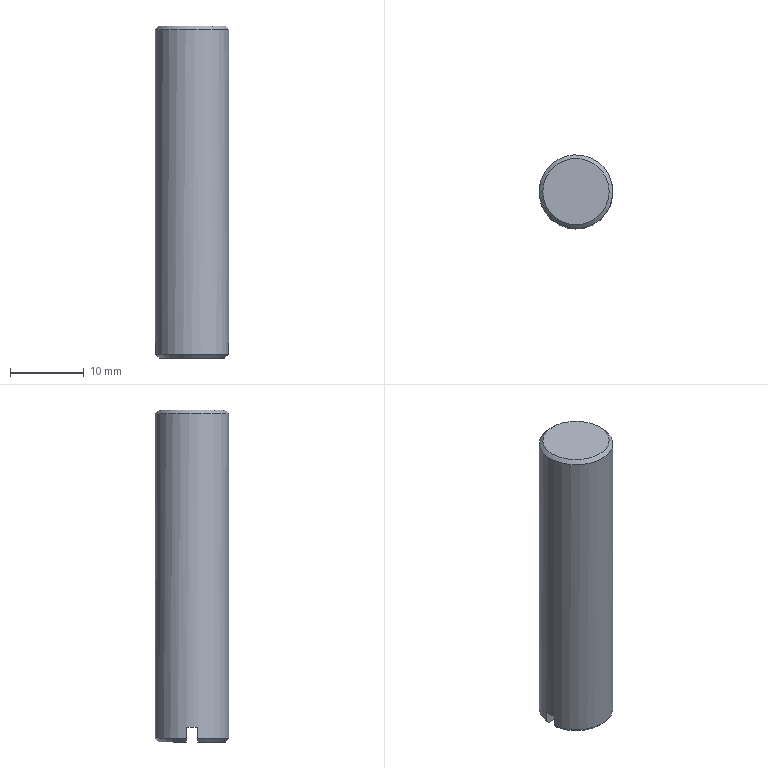Part | NX | 1 solid | 10 faces | box 10 x 10 x 45 mm | volume 3497 mm3 | plane 6 | cone 3 | cylinder 1 | commonest cylinder face diameters 10 x1
STEP:
#1=CARTESIAN_POINT('',(4.437,-0.75,-22.5));
#2=VERTEX_POINT('',#1);
#3=CARTESIAN_POINT('',(-4.437,-0.75,-22.5));
#4=VERTEX_POINT('',#3);
#5=CARTESIAN_POINT('',(0.,0.,-22.5));
#6=DIRECTION('',(0.,0.,1.));
#7=DIRECTION('',(1.,0.,0.));
#8=AXIS2_PLACEMENT_3D('',#5,#6,#7);
#9=CIRCLE('',#8,4.5);
#10=EDGE_CURVE('',#2,#4,#9,.F.);
#11=ORIENTED_EDGE('',*,*,#10,.T.);
#12=CARTESIAN_POINT('',(7.5,-0.75,-22.5));
#13=DIRECTION('',(-1.,0.,0.));
#14=VECTOR('',#13,1000.);
#15=LINE('',#12,#14);
#16=EDGE_CURVE('',#2,#4,#15,.T.);
#17=ORIENTED_EDGE('',*,*,#16,.F.);
#18=EDGE_LOOP('',(#11,#17));
#19=FACE_BOUND('',#18,.T.);
#20=CARTESIAN_POINT('',(0.,0.,-22.5));
#21=DIRECTION('',(0.,0.,1.));
#22=DIRECTION('',(1.,0.,0.));
#23=AXIS2_PLACEMENT_3D('',#20,#21,#22);
#24=PLANE('',#23);
#25=ADVANCED_FACE('',(#19),#24,.F.);
#26=CARTESIAN_POINT('',(4.943,-0.75,-22.));
#27=VERTEX_POINT('',#26);
#28=CARTESIAN_POINT('',(4.943,-0.75,-22.));
#29=CARTESIAN_POINT('',(4.775,-0.75,-22.167));
#30=CARTESIAN_POINT('',(4.606,-0.75,-22.333));
#31=CARTESIAN_POINT('',(4.437,-0.75,-22.5));
#32=B_SPLINE_CURVE_WITH_KNOTS('',3,(#28,#29,#30,#31),.UNSPECIFIED.,.F.,.F.,(4,4),(0.008518,0.00923),.UNSPECIFIED.);
#33=EDGE_CURVE('',#27,#2,#32,.T.);
#34=ORIENTED_EDGE('',*,*,#33,.F.);
#35=CARTESIAN_POINT('',(-4.943,-0.75,-22.));
#36=VERTEX_POINT('',#35);
#37=CARTESIAN_POINT('',(0.,0.,-22.));
#38=DIRECTION('',(0.,0.,1.));
#39=DIRECTION('',(1.,0.,0.));
#40=AXIS2_PLACEMENT_3D('',#37,#38,#39);
#41=CIRCLE('',#40,5.);
#42=EDGE_CURVE('',#36,#27,#41,.T.);
#43=ORIENTED_EDGE('',*,*,#42,.F.);
#44=CARTESIAN_POINT('',(-4.437,-0.75,-22.5));
#45=CARTESIAN_POINT('',(-4.606,-0.75,-22.333));
#46=CARTESIAN_POINT('',(-4.775,-0.75,-22.167));
#47=CARTESIAN_POINT('',(-4.943,-0.75,-22.));
#48=B_SPLINE_CURVE_WITH_KNOTS('',3,(#44,#45,#46,#47),.UNSPECIFIED.,.F.,.F.,(4,4),(0.02102,0.02173),.UNSPECIFIED.);
#49=EDGE_CURVE('',#4,#36,#48,.T.);
#50=ORIENTED_EDGE('',*,*,#49,.F.);
#51=ORIENTED_EDGE('',*,*,#10,.F.);
#52=EDGE_LOOP('',(#34,#43,#50,#51));
#53=FACE_BOUND('',#52,.T.);
#54=CARTESIAN_POINT('',(0.,0.,-22.));
#55=DIRECTION('',(0.,0.,1.));
#56=DIRECTION('',(1.,0.,0.));
#57=AXIS2_PLACEMENT_3D('',#54,#55,#56);
#58=CONICAL_SURFACE('',#57,5.,0.7854);
#59=ADVANCED_FACE('',(#53),#58,.T.);
#60=CARTESIAN_POINT('',(-4.943,0.75,-20.5));
#61=VERTEX_POINT('',#60);
#62=CARTESIAN_POINT('',(-4.943,-0.75,-20.5));
#63=VERTEX_POINT('',#62);
#64=CARTESIAN_POINT('',(0.,0.,-20.5));
#65=DIRECTION('',(0.,0.,1.));
#66=DIRECTION('',(1.,0.,0.));
#67=AXIS2_PLACEMENT_3D('',#64,#65,#66);
#68=CIRCLE('',#67,5.);
#69=EDGE_CURVE('',#61,#63,#68,.T.);
#70=ORIENTED_EDGE('',*,*,#69,.T.);
#71=CARTESIAN_POINT('',(-4.943,-0.75,22.5));
#72=DIRECTION('',(0.,0.,-1.));
#73=VECTOR('',#72,1000.);
#74=LINE('',#71,#73);
#75=EDGE_CURVE('',#63,#36,#74,.T.);
#76=ORIENTED_EDGE('',*,*,#75,.T.);
#77=ORIENTED_EDGE('',*,*,#42,.T.);
#78=CARTESIAN_POINT('',(4.943,-0.75,-20.5));
#79=VERTEX_POINT('',#78);
#80=CARTESIAN_POINT('',(4.943,-0.75,22.5));
#81=DIRECTION('',(0.,0.,-1.));
#82=VECTOR('',#81,1000.);
#83=LINE('',#80,#82);
#84=EDGE_CURVE('',#27,#79,#83,.F.);
#85=ORIENTED_EDGE('',*,*,#84,.T.);
#86=CARTESIAN_POINT('',(4.943,0.75,-20.5));
#87=VERTEX_POINT('',#86);
#88=CARTESIAN_POINT('',(0.,0.,-20.5));
#89=DIRECTION('',(0.,0.,1.));
#90=DIRECTION('',(1.,0.,0.));
#91=AXIS2_PLACEMENT_3D('',#88,#89,#90);
#92=CIRCLE('',#91,5.);
#93=EDGE_CURVE('',#79,#87,#92,.T.);
#94=ORIENTED_EDGE('',*,*,#93,.T.);
#95=CARTESIAN_POINT('',(4.943,0.75,-22.));
#96=VERTEX_POINT('',#95);
#97=CARTESIAN_POINT('',(4.943,0.75,22.5));
#98=DIRECTION('',(0.,0.,-1.));
#99=VECTOR('',#98,1000.);
#100=LINE('',#97,#99);
#101=EDGE_CURVE('',#87,#96,#100,.T.);
#102=ORIENTED_EDGE('',*,*,#101,.T.);
#103=CARTESIAN_POINT('',(-4.943,0.75,-22.));
#104=VERTEX_POINT('',#103);
#105=CARTESIAN_POINT('',(0.,0.,-22.));
#106=DIRECTION('',(0.,0.,1.));
#107=DIRECTION('',(1.,0.,0.));
#108=AXIS2_PLACEMENT_3D('',#105,#106,#107);
#109=CIRCLE('',#108,5.);
#110=EDGE_CURVE('',#96,#104,#109,.T.);
#111=ORIENTED_EDGE('',*,*,#110,.T.);
#112=CARTESIAN_POINT('',(-4.943,0.75,22.5));
#113=DIRECTION('',(0.,0.,-1.));
#114=VECTOR('',#113,1000.);
#115=LINE('',#112,#114);
#116=EDGE_CURVE('',#104,#61,#115,.F.);
#117=ORIENTED_EDGE('',*,*,#116,.T.);
#118=EDGE_LOOP('',(#70,#76,#77,#85,#94,#102,#111,#117));
#119=FACE_BOUND('',#118,.T.);
#120=CARTESIAN_POINT('',(5.,0.,22.));
#121=VERTEX_POINT('',#120);
#122=CARTESIAN_POINT('',(0.,0.,22.));
#123=DIRECTION('',(0.,0.,1.));
#124=DIRECTION('',(1.,0.,0.));
#125=AXIS2_PLACEMENT_3D('',#122,#123,#124);
#126=CIRCLE('',#125,5.);
#127=EDGE_CURVE('',#121,#121,#126,.F.);
#128=ORIENTED_EDGE('',*,*,#127,.T.);
#129=EDGE_LOOP('',(#128));
#130=FACE_BOUND('',#129,.T.);
#131=CARTESIAN_POINT('',(0.,0.,22.5));
#132=DIRECTION('',(0.,0.,-1.));
#133=DIRECTION('',(-1.,0.,0.));
#134=AXIS2_PLACEMENT_3D('',#131,#132,#133);
#135=CYLINDRICAL_SURFACE('',#134,5.);
#136=ADVANCED_FACE('',(#119,#130),#135,.T.);
#137=CARTESIAN_POINT('',(4.5,0.,22.5));
#138=VERTEX_POINT('',#137);
#139=CARTESIAN_POINT('',(0.,0.,22.5));
#140=DIRECTION('',(0.,0.,1.));
#141=DIRECTION('',(1.,0.,0.));
#142=AXIS2_PLACEMENT_3D('',#139,#140,#141);
#143=CIRCLE('',#142,4.5);
#144=EDGE_CURVE('',#138,#138,#143,.T.);
#145=ORIENTED_EDGE('',*,*,#144,.T.);
#146=EDGE_LOOP('',(#145));
#147=FACE_BOUND('',#146,.T.);
#148=CARTESIAN_POINT('',(0.,0.,22.5));
#149=DIRECTION('',(0.,0.,1.));
#150=DIRECTION('',(1.,0.,0.));
#151=AXIS2_PLACEMENT_3D('',#148,#149,#150);
#152=PLANE('',#151);
#153=ADVANCED_FACE('',(#147),#152,.T.);
#154=CARTESIAN_POINT('',(-4.437,0.75,-22.5));
#155=VERTEX_POINT('',#154);
#156=CARTESIAN_POINT('',(4.437,0.75,-22.5));
#157=VERTEX_POINT('',#156);
#158=CARTESIAN_POINT('',(0.,0.,-22.5));
#159=DIRECTION('',(0.,0.,1.));
#160=DIRECTION('',(1.,0.,0.));
#161=AXIS2_PLACEMENT_3D('',#158,#159,#160);
#162=CIRCLE('',#161,4.5);
#163=EDGE_CURVE('',#155,#157,#162,.F.);
#164=ORIENTED_EDGE('',*,*,#163,.T.);
#165=CARTESIAN_POINT('',(7.5,0.75,-22.5));
#166=DIRECTION('',(1.,0.,0.));
#167=VECTOR('',#166,1000.);
#168=LINE('',#165,#167);
#169=EDGE_CURVE('',#155,#157,#168,.T.);
#170=ORIENTED_EDGE('',*,*,#169,.F.);
#171=EDGE_LOOP('',(#164,#170));
#172=FACE_BOUND('',#171,.T.);
#173=CARTESIAN_POINT('',(0.,0.,-22.5));
#174=DIRECTION('',(0.,0.,1.));
#175=DIRECTION('',(1.,0.,0.));
#176=AXIS2_PLACEMENT_3D('',#173,#174,#175);
#177=PLANE('',#176);
#178=ADVANCED_FACE('',(#172),#177,.F.);
#179=CARTESIAN_POINT('',(-4.943,0.75,-22.));
#180=CARTESIAN_POINT('',(-4.775,0.75,-22.167));
#181=CARTESIAN_POINT('',(-4.606,0.75,-22.333));
#182=CARTESIAN_POINT('',(-4.437,0.75,-22.5));
#183=B_SPLINE_CURVE_WITH_KNOTS('',3,(#179,#180,#181,#182),.UNSPECIFIED.,.F.,.F.,(4,4),(0.008518,0.00923),.UNSPECIFIED.);
#184=EDGE_CURVE('',#104,#155,#183,.T.);
#185=ORIENTED_EDGE('',*,*,#184,.F.);
#186=ORIENTED_EDGE('',*,*,#110,.F.);
#187=CARTESIAN_POINT('',(4.437,0.75,-22.5));
#188=CARTESIAN_POINT('',(4.606,0.75,-22.333));
#189=CARTESIAN_POINT('',(4.775,0.75,-22.167));
#190=CARTESIAN_POINT('',(4.943,0.75,-22.));
#191=B_SPLINE_CURVE_WITH_KNOTS('',3,(#187,#188,#189,#190),.UNSPECIFIED.,.F.,.F.,(4,4),(0.02102,0.02173),.UNSPECIFIED.);
#192=EDGE_CURVE('',#157,#96,#191,.T.);
#193=ORIENTED_EDGE('',*,*,#192,.F.);
#194=ORIENTED_EDGE('',*,*,#163,.F.);
#195=EDGE_LOOP('',(#185,#186,#193,#194));
#196=FACE_BOUND('',#195,.T.);
#197=CARTESIAN_POINT('',(0.,0.,-22.));
#198=DIRECTION('',(0.,0.,1.));
#199=DIRECTION('',(1.,0.,0.));
#200=AXIS2_PLACEMENT_3D('',#197,#198,#199);
#201=CONICAL_SURFACE('',#200,5.,0.7854);
#202=ADVANCED_FACE('',(#196),#201,.T.);
#203=ORIENTED_EDGE('',*,*,#127,.F.);
#204=EDGE_LOOP('',(#203));
#205=FACE_BOUND('',#204,.T.);
#206=ORIENTED_EDGE('',*,*,#144,.F.);
#207=EDGE_LOOP('',(#206));
#208=FACE_BOUND('',#207,.T.);
#209=CARTESIAN_POINT('',(0.,0.,22.5));
#210=DIRECTION('',(0.,0.,-1.));
#211=DIRECTION('',(-1.,0.,0.));
#212=AXIS2_PLACEMENT_3D('',#209,#210,#211);
#213=CONICAL_SURFACE('',#212,4.5,0.7854);
#214=ADVANCED_FACE('',(#205,#208),#213,.T.);
#215=CARTESIAN_POINT('',(7.5,0.75,-20.5));
#216=DIRECTION('',(1.,0.,0.));
#217=VECTOR('',#216,1000.);
#218=LINE('',#215,#217);
#219=EDGE_CURVE('',#61,#87,#218,.T.);
#220=ORIENTED_EDGE('',*,*,#219,.T.);
#221=ORIENTED_EDGE('',*,*,#93,.F.);
#222=CARTESIAN_POINT('',(7.5,-0.75,-20.5));
#223=DIRECTION('',(-1.,0.,0.));
#224=VECTOR('',#223,1000.);
#225=LINE('',#222,#224);
#226=EDGE_CURVE('',#79,#63,#225,.T.);
#227=ORIENTED_EDGE('',*,*,#226,.T.);
#228=ORIENTED_EDGE('',*,*,#69,.F.);
#229=EDGE_LOOP('',(#220,#221,#227,#228));
#230=FACE_BOUND('',#229,.T.);
#231=CARTESIAN_POINT('',(0.,0.,-20.5));
#232=DIRECTION('',(0.,0.,1.));
#233=DIRECTION('',(1.,0.,0.));
#234=AXIS2_PLACEMENT_3D('',#231,#232,#233);
#235=PLANE('',#234);
#236=ADVANCED_FACE('',(#230),#235,.F.);
#237=ORIENTED_EDGE('',*,*,#33,.T.);
#238=ORIENTED_EDGE('',*,*,#16,.T.);
#239=ORIENTED_EDGE('',*,*,#49,.T.);
#240=ORIENTED_EDGE('',*,*,#75,.F.);
#241=ORIENTED_EDGE('',*,*,#226,.F.);
#242=ORIENTED_EDGE('',*,*,#84,.F.);
#243=EDGE_LOOP('',(#237,#238,#239,#240,#241,#242));
#244=FACE_BOUND('',#243,.T.);
#245=CARTESIAN_POINT('',(7.5,-0.75,-20.5));
#246=DIRECTION('',(0.,-1.,0.));
#247=DIRECTION('',(0.,0.,-1.));
#248=AXIS2_PLACEMENT_3D('',#245,#246,#247);
#249=PLANE('',#248);
#250=ADVANCED_FACE('',(#244),#249,.F.);
#251=ORIENTED_EDGE('',*,*,#184,.T.);
#252=ORIENTED_EDGE('',*,*,#169,.T.);
#253=ORIENTED_EDGE('',*,*,#192,.T.);
#254=ORIENTED_EDGE('',*,*,#101,.F.);
#255=ORIENTED_EDGE('',*,*,#219,.F.);
#256=ORIENTED_EDGE('',*,*,#116,.F.);
#257=EDGE_LOOP('',(#251,#252,#253,#254,#255,#256));
#258=FACE_BOUND('',#257,.T.);
#259=CARTESIAN_POINT('',(7.5,0.75,-20.5));
#260=DIRECTION('',(0.,1.,0.));
#261=DIRECTION('',(0.,0.,1.));
#262=AXIS2_PLACEMENT_3D('',#259,#260,#261);
#263=PLANE('',#262);
#264=ADVANCED_FACE('',(#258),#263,.F.);
#265=CLOSED_SHELL('',(#25,#59,#136,#153,#178,#202,#214,#236,#250,#264));
#266=MANIFOLD_SOLID_BREP('',#265);
#267=(LENGTH_UNIT()NAMED_UNIT(*)SI_UNIT(.MILLI.,.METRE.));
#268=UNCERTAINTY_MEASURE_WITH_UNIT(LENGTH_MEASURE(0.0508),#267,'','');
#269=(NAMED_UNIT(*)PLANE_ANGLE_UNIT()SI_UNIT($,.RADIAN.));
#270=(NAMED_UNIT(*)SI_UNIT($,.STERADIAN.)SOLID_ANGLE_UNIT());
#271=(GEOMETRIC_REPRESENTATION_CONTEXT(3)GLOBAL_UNCERTAINTY_ASSIGNED_CONTEXT((#268))GLOBAL_UNIT_ASSIGNED_CONTEXT((#267,#269,#270))REPRESENTATION_CONTEXT('',''));
#272=ADVANCED_BREP_SHAPE_REPRESENTATION('',(#266),#271);